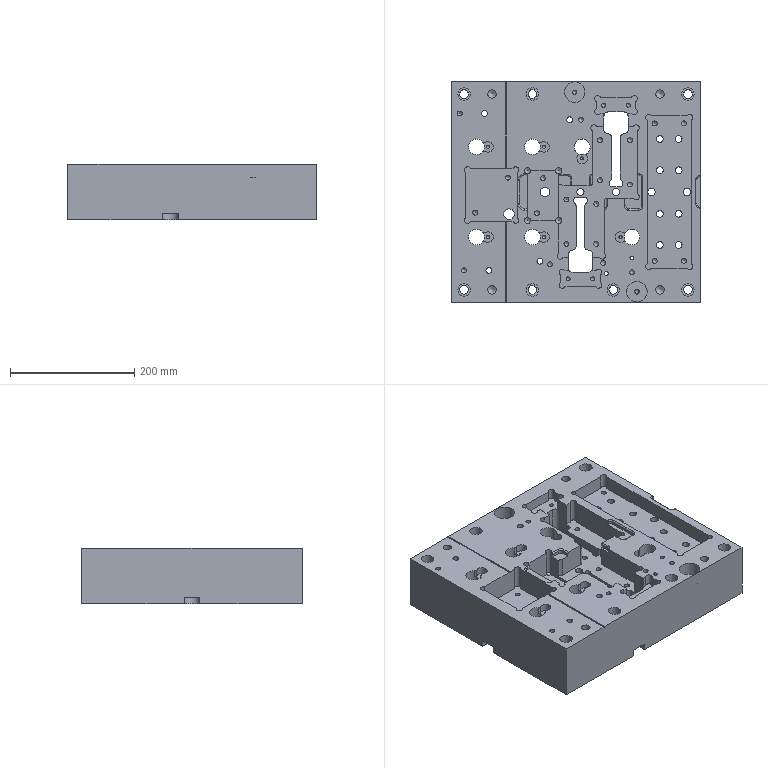Part | STEP file | 1_id126_x_t | 1 solid | 350 faces | box 400 x 355 x 90 mm | volume 10202987 mm3 | cylinder 181 | plane 116 | cone 43 | torus 10 | commonest cylinder face diameters 10 x40 7.938 x22 6 x16 4 x14 11 x12 12 x8